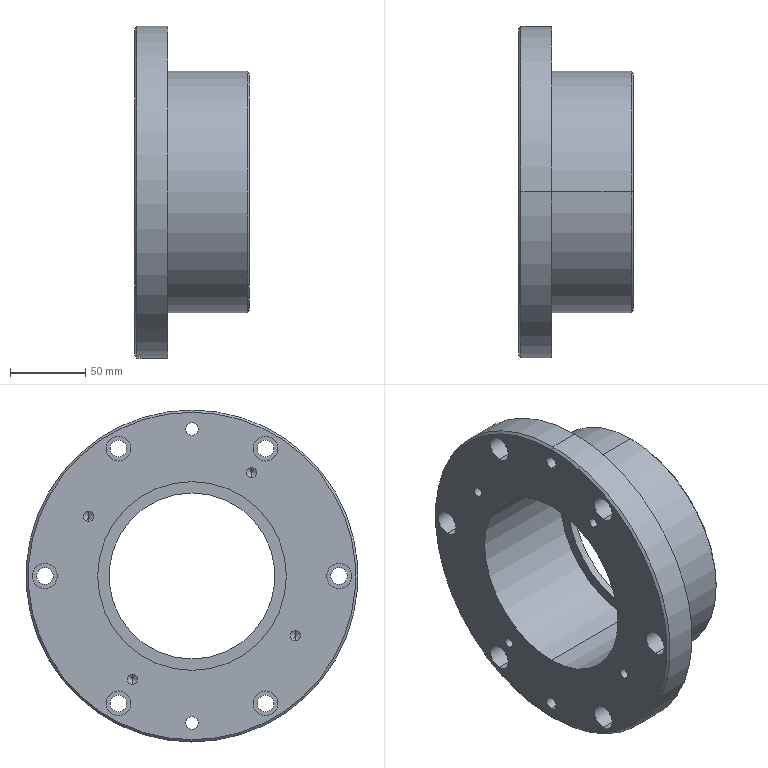Part | STEP file | 46 Spindle Front Sleeve | 1 solid | 66 faces | box 76 x 220 x 220 mm | volume 975565 mm3 | cylinder 44 | cone 12 | plane 10 | commonest cylinder face diameters 11 x12 16.5 x12 6.8 x8 8.5 x4 110 x2 125 x2